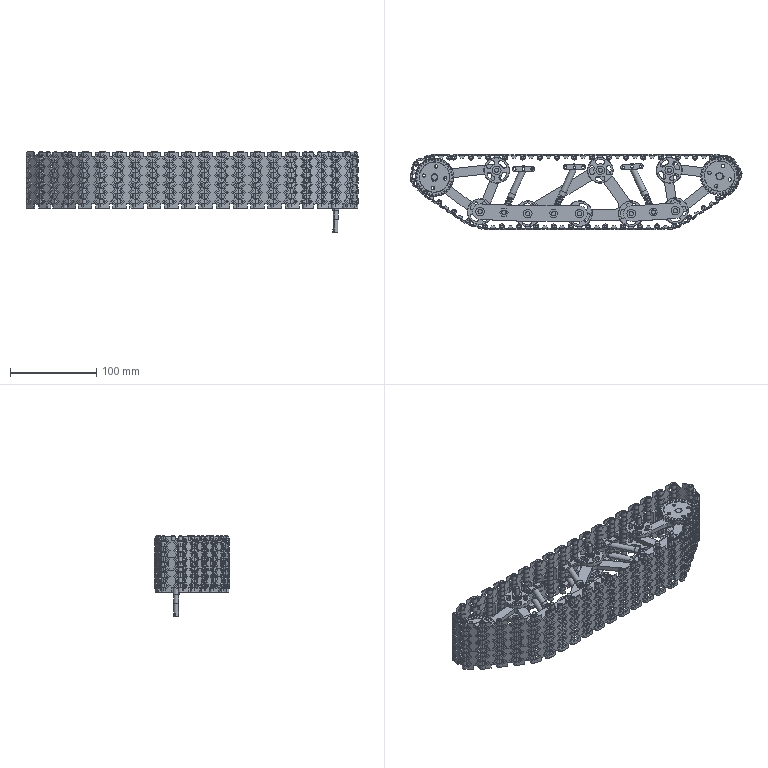Part | SolidWorks | features CompositeCurve 233, ReferencePattern 40, LocalChainPattern 1 | 184 solids | 17119 faces | volume 270065 mm3 | plane 12016 | cylinder 4631 | spline 292 | torus 92 | cone 88 | commonest cylinder face diameters 5.8 x1353 3 x950 1.032 x656 4 x368 2 x256 5 x154